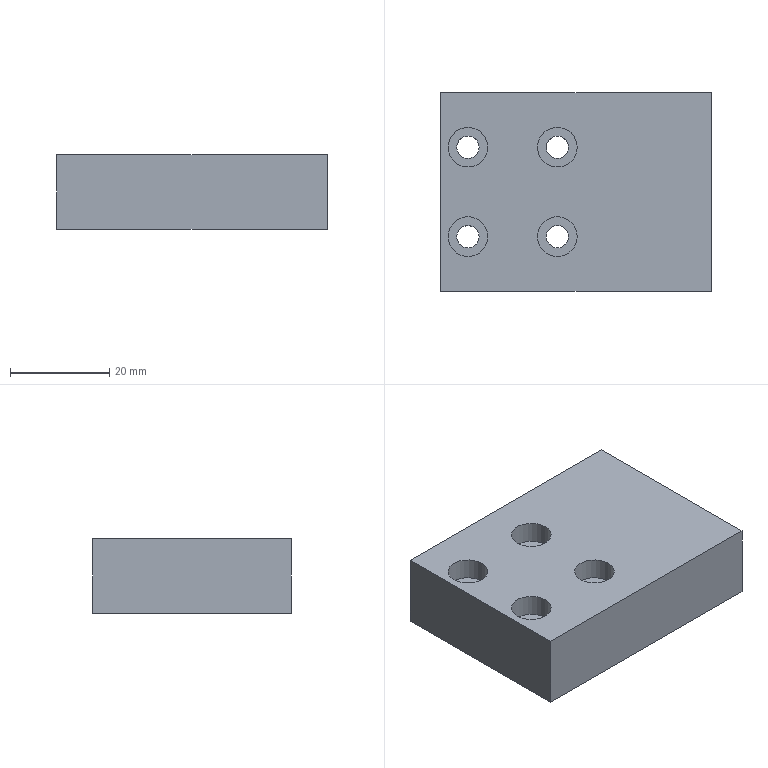Part | NX | features BREP 1 | 1 solid | 28 faces | box 54.5 x 40 x 15 mm | volume 29612 mm3 | cylinder 13 | plane 12 | cone 3 | commonest cylinder face diameters 4.5 x4 6 x4 8 x4 6.8 x1
STEP:
#1=CARTESIAN_POINT('',(-1.5,-9.,3.1));
#2=VERTEX_POINT('',#1);
#3=CARTESIAN_POINT('',(-3.75,-9.,3.1));
#4=DIRECTION('',(0.,0.,1.));
#5=DIRECTION('',(1.,0.,0.));
#6=AXIS2_PLACEMENT_3D('',#3,#4,#5);
#7=CIRCLE('',#6,2.25);
#8=EDGE_CURVE('',#2,#2,#7,.T.);
#9=ORIENTED_EDGE('',*,*,#8,.T.);
#10=EDGE_LOOP('',(#9));
#11=FACE_BOUND('',#10,.T.);
#12=CARTESIAN_POINT('',(-6.,-9.,-4.5));
#13=VERTEX_POINT('',#12);
#14=CARTESIAN_POINT('',(-3.75,-9.,-4.5));
#15=DIRECTION('',(0.,0.,1.));
#16=DIRECTION('',(-1.,0.,0.));
#17=AXIS2_PLACEMENT_3D('',#14,#15,#16);
#18=CIRCLE('',#17,2.25);
#19=EDGE_CURVE('',#13,#13,#18,.T.);
#20=ORIENTED_EDGE('',*,*,#19,.F.);
#21=EDGE_LOOP('',(#20));
#22=FACE_BOUND('',#21,.T.);
#23=CARTESIAN_POINT('',(-3.75,-9.,7.5));
#24=DIRECTION('',(0.,0.,1.));
#25=DIRECTION('',(-1.,0.,0.));
#26=AXIS2_PLACEMENT_3D('',#23,#24,#25);
#27=CYLINDRICAL_SURFACE('',#26,2.25);
#28=ADVANCED_FACE('',(#11,#22),#27,.F.);
#29=CARTESIAN_POINT('',(-19.5,9.,3.1));
#30=VERTEX_POINT('',#29);
#31=CARTESIAN_POINT('',(-21.75,9.,3.1));
#32=DIRECTION('',(0.,0.,1.));
#33=DIRECTION('',(1.,0.,0.));
#34=AXIS2_PLACEMENT_3D('',#31,#32,#33);
#35=CIRCLE('',#34,2.25);
#36=EDGE_CURVE('',#30,#30,#35,.T.);
#37=ORIENTED_EDGE('',*,*,#36,.T.);
#38=EDGE_LOOP('',(#37));
#39=FACE_BOUND('',#38,.T.);
#40=CARTESIAN_POINT('',(-24.,9.,-4.5));
#41=VERTEX_POINT('',#40);
#42=CARTESIAN_POINT('',(-21.75,9.,-4.5));
#43=DIRECTION('',(0.,0.,1.));
#44=DIRECTION('',(-1.,0.,0.));
#45=AXIS2_PLACEMENT_3D('',#42,#43,#44);
#46=CIRCLE('',#45,2.25);
#47=EDGE_CURVE('',#41,#41,#46,.T.);
#48=ORIENTED_EDGE('',*,*,#47,.F.);
#49=EDGE_LOOP('',(#48));
#50=FACE_BOUND('',#49,.T.);
#51=CARTESIAN_POINT('',(-21.75,9.,7.5));
#52=DIRECTION('',(0.,0.,1.));
#53=DIRECTION('',(-1.,0.,0.));
#54=AXIS2_PLACEMENT_3D('',#51,#52,#53);
#55=CYLINDRICAL_SURFACE('',#54,2.25);
#56=ADVANCED_FACE('',(#39,#50),#55,.F.);
#57=CARTESIAN_POINT('',(27.25,0.,-3.4));
#58=VERTEX_POINT('',#57);
#59=CARTESIAN_POINT('',(27.25,0.,0.));
#60=DIRECTION('',(1.,0.,0.));
#61=DIRECTION('',(0.,0.,-1.));
#62=AXIS2_PLACEMENT_3D('',#59,#60,#61);
#63=CIRCLE('',#62,3.4);
#64=EDGE_CURVE('',#58,#58,#63,.T.);
#65=ORIENTED_EDGE('',*,*,#64,.F.);
#66=EDGE_LOOP('',(#65));
#67=FACE_BOUND('',#66,.T.);
#68=CARTESIAN_POINT('',(27.25,15.,-3.));
#69=VERTEX_POINT('',#68);
#70=CARTESIAN_POINT('',(27.25,15.,0.));
#71=DIRECTION('',(1.,0.,0.));
#72=DIRECTION('',(0.,0.,-1.));
#73=AXIS2_PLACEMENT_3D('',#70,#71,#72);
#74=CIRCLE('',#73,3.);
#75=EDGE_CURVE('',#69,#69,#74,.T.);
#76=ORIENTED_EDGE('',*,*,#75,.F.);
#77=EDGE_LOOP('',(#76));
#78=FACE_BOUND('',#77,.T.);
#79=CARTESIAN_POINT('',(27.25,-15.,-3.));
#80=VERTEX_POINT('',#79);
#81=CARTESIAN_POINT('',(27.25,-15.,0.));
#82=DIRECTION('',(1.,0.,0.));
#83=DIRECTION('',(0.,0.,-1.));
#84=AXIS2_PLACEMENT_3D('',#81,#82,#83);
#85=CIRCLE('',#84,3.);
#86=EDGE_CURVE('',#80,#80,#85,.T.);
#87=ORIENTED_EDGE('',*,*,#86,.F.);
#88=EDGE_LOOP('',(#87));
#89=FACE_BOUND('',#88,.T.);
#90=CARTESIAN_POINT('',(27.25,-20.,-7.5));
#91=VERTEX_POINT('',#90);
#92=CARTESIAN_POINT('',(27.25,20.,-7.5));
#93=VERTEX_POINT('',#92);
#94=CARTESIAN_POINT('',(27.25,-20.,-7.5));
#95=DIRECTION('',(0.,1.,0.));
#96=VECTOR('',#95,1000.);
#97=LINE('',#94,#96);
#98=EDGE_CURVE('',#91,#93,#97,.T.);
#99=ORIENTED_EDGE('',*,*,#98,.T.);
#100=CARTESIAN_POINT('',(27.25,20.,7.5));
#101=VERTEX_POINT('',#100);
#102=CARTESIAN_POINT('',(27.25,20.,7.5));
#103=DIRECTION('',(0.,0.,-1.));
#104=VECTOR('',#103,1000.);
#105=LINE('',#102,#104);
#106=EDGE_CURVE('',#101,#93,#105,.T.);
#107=ORIENTED_EDGE('',*,*,#106,.F.);
#108=CARTESIAN_POINT('',(27.25,-20.,7.5));
#109=VERTEX_POINT('',#108);
#110=CARTESIAN_POINT('',(27.25,-20.,7.5));
#111=DIRECTION('',(0.,1.,0.));
#112=VECTOR('',#111,1000.);
#113=LINE('',#110,#112);
#114=EDGE_CURVE('',#109,#101,#113,.T.);
#115=ORIENTED_EDGE('',*,*,#114,.F.);
#116=CARTESIAN_POINT('',(27.25,-20.,7.5));
#117=DIRECTION('',(0.,0.,-1.));
#118=VECTOR('',#117,1000.);
#119=LINE('',#116,#118);
#120=EDGE_CURVE('',#109,#91,#119,.T.);
#121=ORIENTED_EDGE('',*,*,#120,.T.);
#122=EDGE_LOOP('',(#99,#107,#115,#121));
#123=FACE_BOUND('',#122,.T.);
#124=CARTESIAN_POINT('',(27.25,-20.,7.5));
#125=DIRECTION('',(-1.,0.,0.));
#126=DIRECTION('',(0.,0.,-1.));
#127=AXIS2_PLACEMENT_3D('',#124,#125,#126);
#128=PLANE('',#127);
#129=ADVANCED_FACE('',(#67,#78,#89,#123),#128,.F.);
#130=CARTESIAN_POINT('',(-27.25,20.,-7.5));
#131=VERTEX_POINT('',#130);
#132=CARTESIAN_POINT('',(-27.25,20.,-7.5));
#133=DIRECTION('',(-1.,0.,0.));
#134=VECTOR('',#133,1000.);
#135=LINE('',#132,#134);
#136=EDGE_CURVE('',#93,#131,#135,.T.);
#137=ORIENTED_EDGE('',*,*,#136,.T.);
#138=CARTESIAN_POINT('',(-27.25,20.,7.5));
#139=VERTEX_POINT('',#138);
#140=CARTESIAN_POINT('',(-27.25,20.,7.5));
#141=DIRECTION('',(0.,0.,-1.));
#142=VECTOR('',#141,1000.);
#143=LINE('',#140,#142);
#144=EDGE_CURVE('',#139,#131,#143,.T.);
#145=ORIENTED_EDGE('',*,*,#144,.F.);
#146=CARTESIAN_POINT('',(-27.25,20.,7.5));
#147=DIRECTION('',(-1.,0.,0.));
#148=VECTOR('',#147,1000.);
#149=LINE('',#146,#148);
#150=EDGE_CURVE('',#101,#139,#149,.T.);
#151=ORIENTED_EDGE('',*,*,#150,.F.);
#152=ORIENTED_EDGE('',*,*,#106,.T.);
#153=EDGE_LOOP('',(#137,#145,#151,#152));
#154=FACE_BOUND('',#153,.T.);
#155=CARTESIAN_POINT('',(-27.25,20.,7.5));
#156=DIRECTION('',(0.,-1.,0.));
#157=DIRECTION('',(0.,0.,1.));
#158=AXIS2_PLACEMENT_3D('',#155,#156,#157);
#159=PLANE('',#158);
#160=ADVANCED_FACE('',(#154),#159,.F.);
#161=CARTESIAN_POINT('',(-27.25,-20.,-7.5));
#162=VERTEX_POINT('',#161);
#163=CARTESIAN_POINT('',(-27.25,-20.,-7.5));
#164=DIRECTION('',(0.,-1.,0.));
#165=VECTOR('',#164,1000.);
#166=LINE('',#163,#165);
#167=EDGE_CURVE('',#131,#162,#166,.T.);
#168=ORIENTED_EDGE('',*,*,#167,.T.);
#169=CARTESIAN_POINT('',(-27.25,-20.,7.5));
#170=VERTEX_POINT('',#169);
#171=CARTESIAN_POINT('',(-27.25,-20.,7.5));
#172=DIRECTION('',(0.,0.,-1.));
#173=VECTOR('',#172,1000.);
#174=LINE('',#171,#173);
#175=EDGE_CURVE('',#170,#162,#174,.T.);
#176=ORIENTED_EDGE('',*,*,#175,.F.);
#177=CARTESIAN_POINT('',(-27.25,-20.,7.5));
#178=DIRECTION('',(0.,-1.,0.));
#179=VECTOR('',#178,1000.);
#180=LINE('',#177,#179);
#181=EDGE_CURVE('',#139,#170,#180,.T.);
#182=ORIENTED_EDGE('',*,*,#181,.F.);
#183=ORIENTED_EDGE('',*,*,#144,.T.);
#184=EDGE_LOOP('',(#168,#176,#182,#183));
#185=FACE_BOUND('',#184,.T.);
#186=CARTESIAN_POINT('',(-27.25,-20.,7.5));
#187=DIRECTION('',(1.,0.,0.));
#188=DIRECTION('',(0.,0.,1.));
#189=AXIS2_PLACEMENT_3D('',#186,#187,#188);
#190=PLANE('',#189);
#191=ADVANCED_FACE('',(#185),#190,.F.);
#192=CARTESIAN_POINT('',(-27.25,-20.,-7.5));
#193=DIRECTION('',(1.,0.,0.));
#194=VECTOR('',#193,1000.);
#195=LINE('',#192,#194);
#196=EDGE_CURVE('',#162,#91,#195,.T.);
#197=ORIENTED_EDGE('',*,*,#196,.T.);
#198=ORIENTED_EDGE('',*,*,#120,.F.);
#199=CARTESIAN_POINT('',(-27.25,-20.,7.5));
#200=DIRECTION('',(1.,0.,0.));
#201=VECTOR('',#200,1000.);
#202=LINE('',#199,#201);
#203=EDGE_CURVE('',#170,#109,#202,.T.);
#204=ORIENTED_EDGE('',*,*,#203,.F.);
#205=ORIENTED_EDGE('',*,*,#175,.T.);
#206=EDGE_LOOP('',(#197,#198,#204,#205));
#207=FACE_BOUND('',#206,.T.);
#208=CARTESIAN_POINT('',(-27.25,-20.,7.5));
#209=DIRECTION('',(0.,1.,0.));
#210=DIRECTION('',(0.,0.,-1.));
#211=AXIS2_PLACEMENT_3D('',#208,#209,#210);
#212=PLANE('',#211);
#213=ADVANCED_FACE('',(#207),#212,.F.);
#214=CARTESIAN_POINT('',(-17.75,9.,7.5));
#215=VERTEX_POINT('',#214);
#216=CARTESIAN_POINT('',(-21.75,9.,7.5));
#217=DIRECTION('',(0.,0.,1.));
#218=DIRECTION('',(1.,0.,0.));
#219=AXIS2_PLACEMENT_3D('',#216,#217,#218);
#220=CIRCLE('',#219,4.);
#221=EDGE_CURVE('',#215,#215,#220,.T.);
#222=ORIENTED_EDGE('',*,*,#221,.F.);
#223=EDGE_LOOP('',(#222));
#224=FACE_BOUND('',#223,.T.);
#225=CARTESIAN_POINT('',(0.25,-9.,7.5));
#226=VERTEX_POINT('',#225);
#227=CARTESIAN_POINT('',(-3.75,-9.,7.5));
#228=DIRECTION('',(0.,0.,1.));
#229=DIRECTION('',(1.,0.,0.));
#230=AXIS2_PLACEMENT_3D('',#227,#228,#229);
#231=CIRCLE('',#230,4.);
#232=EDGE_CURVE('',#226,#226,#231,.T.);
#233=ORIENTED_EDGE('',*,*,#232,.F.);
#234=EDGE_LOOP('',(#233));
#235=FACE_BOUND('',#234,.T.);
#236=CARTESIAN_POINT('',(-17.75,-9.,7.5));
#237=VERTEX_POINT('',#236);
#238=CARTESIAN_POINT('',(-21.75,-9.,7.5));
#239=DIRECTION('',(0.,0.,1.));
#240=DIRECTION('',(1.,0.,0.));
#241=AXIS2_PLACEMENT_3D('',#238,#239,#240);
#242=CIRCLE('',#241,4.);
#243=EDGE_CURVE('',#237,#237,#242,.T.);
#244=ORIENTED_EDGE('',*,*,#243,.F.);
#245=EDGE_LOOP('',(#244));
#246=FACE_BOUND('',#245,.T.);
#247=CARTESIAN_POINT('',(0.25,9.,7.5));
#248=VERTEX_POINT('',#247);
#249=CARTESIAN_POINT('',(-3.75,9.,7.5));
#250=DIRECTION('',(0.,0.,1.));
#251=DIRECTION('',(1.,0.,0.));
#252=AXIS2_PLACEMENT_3D('',#249,#250,#251);
#253=CIRCLE('',#252,4.);
#254=EDGE_CURVE('',#248,#248,#253,.T.);
#255=ORIENTED_EDGE('',*,*,#254,.F.);
#256=EDGE_LOOP('',(#255));
#257=FACE_BOUND('',#256,.T.);
#258=ORIENTED_EDGE('',*,*,#114,.T.);
#259=ORIENTED_EDGE('',*,*,#150,.T.);
#260=ORIENTED_EDGE('',*,*,#181,.T.);
#261=ORIENTED_EDGE('',*,*,#203,.T.);
#262=EDGE_LOOP('',(#258,#259,#260,#261));
#263=FACE_BOUND('',#262,.T.);
#264=CARTESIAN_POINT('',(0.,0.,7.5));
#265=DIRECTION('',(0.,0.,-1.));
#266=DIRECTION('',(1.,0.,0.));
#267=AXIS2_PLACEMENT_3D('',#264,#265,#266);
#268=PLANE('',#267);
#269=ADVANCED_FACE('',(#224,#235,#246,#257,#263),#268,.F.);
#270=CARTESIAN_POINT('',(-24.75,9.,-7.5));
#271=VERTEX_POINT('',#270);
#272=CARTESIAN_POINT('',(-21.75,9.,-7.5));
#273=DIRECTION('',(0.,0.,-1.));
#274=DIRECTION('',(-1.,0.,0.));
#275=AXIS2_PLACEMENT_3D('',#272,#273,#274);
#276=CIRCLE('',#275,3.);
#277=EDGE_CURVE('',#271,#271,#276,.T.);
#278=ORIENTED_EDGE('',*,*,#277,.F.);
#279=EDGE_LOOP('',(#278));
#280=FACE_BOUND('',#279,.T.);
#281=CARTESIAN_POINT('',(-6.75,-9.,-7.5));
#282=VERTEX_POINT('',#281);
#283=CARTESIAN_POINT('',(-3.75,-9.,-7.5));
#284=DIRECTION('',(0.,0.,-1.));
#285=DIRECTION('',(-1.,0.,0.));
#286=AXIS2_PLACEMENT_3D('',#283,#284,#285);
#287=CIRCLE('',#286,3.);
#288=EDGE_CURVE('',#282,#282,#287,.T.);
#289=ORIENTED_EDGE('',*,*,#288,.F.);
#290=EDGE_LOOP('',(#289));
#291=FACE_BOUND('',#290,.T.);
#292=CARTESIAN_POINT('',(-19.5,-9.,-7.5));
#293=VERTEX_POINT('',#292);
#294=CARTESIAN_POINT('',(-21.75,-9.,-7.5));
#295=DIRECTION('',(0.,0.,1.));
#296=DIRECTION('',(1.,0.,0.));
#297=AXIS2_PLACEMENT_3D('',#294,#295,#296);
#298=CIRCLE('',#297,2.25);
#299=EDGE_CURVE('',#293,#293,#298,.T.);
#300=ORIENTED_EDGE('',*,*,#299,.T.);
#301=EDGE_LOOP('',(#300));
#302=FACE_BOUND('',#301,.T.);
#303=CARTESIAN_POINT('',(-1.5,9.,-7.5));
#304=VERTEX_POINT('',#303);
#305=CARTESIAN_POINT('',(-3.75,9.,-7.5));
#306=DIRECTION('',(0.,0.,1.));
#307=DIRECTION('',(1.,0.,0.));
#308=AXIS2_PLACEMENT_3D('',#305,#306,#307);
#309=CIRCLE('',#308,2.25);
#310=EDGE_CURVE('',#304,#304,#309,.T.);
#311=ORIENTED_EDGE('',*,*,#310,.T.);
#312=EDGE_LOOP('',(#311));
#313=FACE_BOUND('',#312,.T.);
#314=ORIENTED_EDGE('',*,*,#98,.F.);
#315=ORIENTED_EDGE('',*,*,#196,.F.);
#316=ORIENTED_EDGE('',*,*,#167,.F.);
#317=ORIENTED_EDGE('',*,*,#136,.F.);
#318=EDGE_LOOP('',(#314,#315,#316,#317));
#319=FACE_BOUND('',#318,.T.);
#320=CARTESIAN_POINT('',(0.,0.,-7.5));
#321=DIRECTION('',(0.,0.,-1.));
#322=DIRECTION('',(1.,0.,0.));
#323=AXIS2_PLACEMENT_3D('',#320,#321,#322);
#324=PLANE('',#323);
#325=ADVANCED_FACE('',(#280,#291,#302,#313,#319),#324,.T.);
#326=ORIENTED_EDGE('',*,*,#310,.F.);
#327=EDGE_LOOP('',(#326));
#328=FACE_BOUND('',#327,.T.);
#329=CARTESIAN_POINT('',(-1.5,9.,3.1));
#330=VERTEX_POINT('',#329);
#331=CARTESIAN_POINT('',(-3.75,9.,3.1));
#332=DIRECTION('',(0.,0.,1.));
#333=DIRECTION('',(1.,0.,0.));
#334=AXIS2_PLACEMENT_3D('',#331,#332,#333);
#335=CIRCLE('',#334,2.25);
#336=EDGE_CURVE('',#330,#330,#335,.T.);
#337=ORIENTED_EDGE('',*,*,#336,.T.);
#338=EDGE_LOOP('',(#337));
#339=FACE_BOUND('',#338,.T.);
#340=CARTESIAN_POINT('',(-3.75,9.,7.5));
#341=DIRECTION('',(0.,0.,1.));
#342=DIRECTION('',(-1.,0.,0.));
#343=AXIS2_PLACEMENT_3D('',#340,#341,#342);
#344=CYLINDRICAL_SURFACE('',#343,2.25);
#345=ADVANCED_FACE('',(#328,#339),#344,.F.);
#346=ORIENTED_EDGE('',*,*,#336,.F.);
#347=EDGE_LOOP('',(#346));
#348=FACE_BOUND('',#347,.T.);
#349=CARTESIAN_POINT('',(0.25,9.,3.1));
#350=VERTEX_POINT('',#349);
#351=CARTESIAN_POINT('',(-3.75,9.,3.1));
#352=DIRECTION('',(0.,0.,1.));
#353=DIRECTION('',(1.,0.,0.));
#354=AXIS2_PLACEMENT_3D('',#351,#352,#353);
#355=CIRCLE('',#354,4.);
#356=EDGE_CURVE('',#350,#350,#355,.T.);
#357=ORIENTED_EDGE('',*,*,#356,.T.);
#358=EDGE_LOOP('',(#357));
#359=FACE_BOUND('',#358,.T.);
#360=CARTESIAN_POINT('',(-1.5,9.,3.1));
#361=DIRECTION('',(0.,0.,-1.));
#362=DIRECTION('',(1.,0.,0.));
#363=AXIS2_PLACEMENT_3D('',#360,#361,#362);
#364=PLANE('',#363);
#365=ADVANCED_FACE('',(#348,#359),#364,.F.);
#366=ORIENTED_EDGE('',*,*,#356,.F.);
#367=EDGE_LOOP('',(#366));
#368=FACE_BOUND('',#367,.T.);
#369=ORIENTED_EDGE('',*,*,#254,.T.);
#370=EDGE_LOOP('',(#369));
#371=FACE_BOUND('',#370,.T.);
#372=CARTESIAN_POINT('',(-3.75,9.,7.5));
#373=DIRECTION('',(0.,0.,1.));
#374=DIRECTION('',(-1.,0.,0.));
#375=AXIS2_PLACEMENT_3D('',#372,#373,#374);
#376=CYLINDRICAL_SURFACE('',#375,4.);
#377=ADVANCED_FACE('',(#368,#371),#376,.F.);
#378=ORIENTED_EDGE('',*,*,#299,.F.);
#379=EDGE_LOOP('',(#378));
#380=FACE_BOUND('',#379,.T.);
#381=CARTESIAN_POINT('',(-19.5,-9.,3.1));
#382=VERTEX_POINT('',#381);
#383=CARTESIAN_POINT('',(-21.75,-9.,3.1));
#384=DIRECTION('',(0.,0.,1.));
#385=DIRECTION('',(1.,0.,0.));
#386=AXIS2_PLACEMENT_3D('',#383,#384,#385);
#387=CIRCLE('',#386,2.25);
#388=EDGE_CURVE('',#382,#382,#387,.T.);
#389=ORIENTED_EDGE('',*,*,#388,.T.);
#390=EDGE_LOOP('',(#389));
#391=FACE_BOUND('',#390,.T.);
#392=CARTESIAN_POINT('',(-21.75,-9.,7.5));
#393=DIRECTION('',(0.,0.,1.));
#394=DIRECTION('',(-1.,0.,0.));
#395=AXIS2_PLACEMENT_3D('',#392,#393,#394);
#396=CYLINDRICAL_SURFACE('',#395,2.25);
#397=ADVANCED_FACE('',(#380,#391),#396,.F.);
#398=ORIENTED_EDGE('',*,*,#388,.F.);
#399=EDGE_LOOP('',(#398));
#400=FACE_BOUND('',#399,.T.);
#401=CARTESIAN_POINT('',(-17.75,-9.,3.1));
#402=VERTEX_POINT('',#401);
#403=CARTESIAN_POINT('',(-21.75,-9.,3.1));
#404=DIRECTION('',(0.,0.,1.));
#405=DIRECTION('',(1.,0.,0.));
#406=AXIS2_PLACEMENT_3D('',#403,#404,#405);
#407=CIRCLE('',#406,4.);
#408=EDGE_CURVE('',#402,#402,#407,.T.);
#409=ORIENTED_EDGE('',*,*,#408,.T.);
#410=EDGE_LOOP('',(#409));
#411=FACE_BOUND('',#410,.T.);
#412=CARTESIAN_POINT('',(-19.5,-9.,3.1));
#413=DIRECTION('',(0.,0.,-1.));
#414=DIRECTION('',(1.,0.,0.));
#415=AXIS2_PLACEMENT_3D('',#412,#413,#414);
#416=PLANE('',#415);
#417=ADVANCED_FACE('',(#400,#411),#416,.F.);
#418=ORIENTED_EDGE('',*,*,#408,.F.);
#419=EDGE_LOOP('',(#418));
#420=FACE_BOUND('',#419,.T.);
#421=ORIENTED_EDGE('',*,*,#243,.T.);
#422=EDGE_LOOP('',(#421));
#423=FACE_BOUND('',#422,.T.);
#424=CARTESIAN_POINT('',(-21.75,-9.,7.5));
#425=DIRECTION('',(0.,0.,1.));
#426=DIRECTION('',(-1.,0.,0.));
#427=AXIS2_PLACEMENT_3D('',#424,#425,#426);
#428=CYLINDRICAL_SURFACE('',#427,4.);
#429=ADVANCED_FACE('',(#420,#423),#428,.F.);
#430=ORIENTED_EDGE('',*,*,#8,.F.);
#431=EDGE_LOOP('',(#430));
#432=FACE_BOUND('',#431,.T.);
#433=CARTESIAN_POINT('',(0.25,-9.,3.1));
#434=VERTEX_POINT('',#433);
#435=CARTESIAN_POINT('',(-3.75,-9.,3.1));
#436=DIRECTION('',(0.,0.,1.));
#437=DIRECTION('',(1.,0.,0.));
#438=AXIS2_PLACEMENT_3D('',#435,#436,#437);
#439=CIRCLE('',#438,4.);
#440=EDGE_CURVE('',#434,#434,#439,.T.);
#441=ORIENTED_EDGE('',*,*,#440,.T.);
#442=EDGE_LOOP('',(#441));
#443=FACE_BOUND('',#442,.T.);
#444=CARTESIAN_POINT('',(-1.5,-9.,3.1));
#445=DIRECTION('',(0.,0.,-1.));
#446=DIRECTION('',(1.,0.,0.));
#447=AXIS2_PLACEMENT_3D('',#444,#445,#446);
#448=PLANE('',#447);
#449=ADVANCED_FACE('',(#432,#443),#448,.F.);
#450=ORIENTED_EDGE('',*,*,#440,.F.);
#451=EDGE_LOOP('',(#450));
#452=FACE_BOUND('',#451,.T.);
#453=ORIENTED_EDGE('',*,*,#232,.T.);
#454=EDGE_LOOP('',(#453));
#455=FACE_BOUND('',#454,.T.);
#456=CARTESIAN_POINT('',(-3.75,-9.,7.5));
#457=DIRECTION('',(0.,0.,1.));
#458=DIRECTION('',(-1.,0.,0.));
#459=AXIS2_PLACEMENT_3D('',#456,#457,#458);
#460=CYLINDRICAL_SURFACE('',#459,4.);
#461=ADVANCED_FACE('',(#452,#455),#460,.F.);
#462=ORIENTED_EDGE('',*,*,#36,.F.);
#463=EDGE_LOOP('',(#462));
#464=FACE_BOUND('',#463,.T.);
#465=CARTESIAN_POINT('',(-17.75,9.,3.1));
#466=VERTEX_POINT('',#465);
#467=CARTESIAN_POINT('',(-21.75,9.,3.1));
#468=DIRECTION('',(0.,0.,1.));
#469=DIRECTION('',(1.,0.,0.));
#470=AXIS2_PLACEMENT_3D('',#467,#468,#469);
#471=CIRCLE('',#470,4.);
#472=EDGE_CURVE('',#466,#466,#471,.T.);
#473=ORIENTED_EDGE('',*,*,#472,.T.);
#474=EDGE_LOOP('',(#473));
#475=FACE_BOUND('',#474,.T.);
#476=CARTESIAN_POINT('',(-19.5,9.,3.1));
#477=DIRECTION('',(0.,0.,-1.));
#478=DIRECTION('',(1.,0.,0.));
#479=AXIS2_PLACEMENT_3D('',#476,#477,#478);
#480=PLANE('',#479);
#481=ADVANCED_FACE('',(#464,#475),#480,.F.);
#482=ORIENTED_EDGE('',*,*,#472,.F.);
#483=EDGE_LOOP('',(#482));
#484=FACE_BOUND('',#483,.T.);
#485=ORIENTED_EDGE('',*,*,#221,.T.);
#486=EDGE_LOOP('',(#485));
#487=FACE_BOUND('',#486,.T.);
#488=CARTESIAN_POINT('',(-21.75,9.,7.5));
#489=DIRECTION('',(0.,0.,1.));
#490=DIRECTION('',(-1.,0.,0.));
#491=AXIS2_PLACEMENT_3D('',#488,#489,#490);
#492=CYLINDRICAL_SURFACE('',#491,4.);
#493=ADVANCED_FACE('',(#484,#487),#492,.F.);
#494=CARTESIAN_POINT('',(13.447,-15.,0.));
#495=VERTEX_POINT('',#494);
#496=VERTEX_LOOP('',#495);
#497=FACE_BOUND('',#496,.T.);
#498=CARTESIAN_POINT('',(15.25,-15.,-3.));
#499=VERTEX_POINT('',#498);
#500=CARTESIAN_POINT('',(15.25,-15.,0.));
#501=DIRECTION('',(1.,0.,0.));
#502=DIRECTION('',(0.,0.,-1.));
#503=AXIS2_PLACEMENT_3D('',#500,#501,#502);
#504=CIRCLE('',#503,3.);
#505=EDGE_CURVE('',#499,#499,#504,.T.);
#506=ORIENTED_EDGE('',*,*,#505,.T.);
#507=EDGE_LOOP('',(#506));
#508=FACE_BOUND('',#507,.T.);
#509=CARTESIAN_POINT('',(15.25,-15.,0.));
#510=DIRECTION('',(1.,0.,0.));
#511=DIRECTION('',(0.,0.,1.));
#512=AXIS2_PLACEMENT_3D('',#509,#510,#511);
#513=CONICAL_SURFACE('',#512,3.,1.03);
#514=ADVANCED_FACE('',(#497,#508),#513,.F.);
#515=ORIENTED_EDGE('',*,*,#505,.F.);
#516=EDGE_LOOP('',(#515));
#517=FACE_BOUND('',#516,.T.);
#518=ORIENTED_EDGE('',*,*,#86,.T.);
#519=EDGE_LOOP('',(#518));
#520=FACE_BOUND('',#519,.T.);
#521=CARTESIAN_POINT('',(27.25,-15.,0.));
#522=DIRECTION('',(1.,0.,0.));
#523=DIRECTION('',(0.,0.,1.));
#524=AXIS2_PLACEMENT_3D('',#521,#522,#523);
#525=CYLINDRICAL_SURFACE('',#524,3.);
#526=ADVANCED_FACE('',(#517,#520),#525,.F.);
#527=CARTESIAN_POINT('',(13.447,15.,0.));
#528=VERTEX_POINT('',#527);
#529=VERTEX_LOOP('',#528);
#530=FACE_BOUND('',#529,.T.);
#531=CARTESIAN_POINT('',(15.25,15.,-3.));
#532=VERTEX_POINT('',#531);
#533=CARTESIAN_POINT('',(15.25,15.,0.));
#534=DIRECTION('',(1.,0.,0.));
#535=DIRECTION('',(0.,0.,-1.));
#536=AXIS2_PLACEMENT_3D('',#533,#534,#535);
#537=CIRCLE('',#536,3.);
#538=EDGE_CURVE('',#532,#532,#537,.T.);
#539=ORIENTED_EDGE('',*,*,#538,.T.);
#540=EDGE_LOOP('',(#539));
#541=FACE_BOUND('',#540,.T.);
#542=CARTESIAN_POINT('',(15.25,15.,0.));
#543=DIRECTION('',(1.,0.,0.));
#544=DIRECTION('',(0.,0.,1.));
#545=AXIS2_PLACEMENT_3D('',#542,#543,#544);
#546=CONICAL_SURFACE('',#545,3.,1.03);
#547=ADVANCED_FACE('',(#530,#541),#546,.F.);
#548=ORIENTED_EDGE('',*,*,#538,.F.);
#549=EDGE_LOOP('',(#548));
#550=FACE_BOUND('',#549,.T.);
#551=ORIENTED_EDGE('',*,*,#75,.T.);
#552=EDGE_LOOP('',(#551));
#553=FACE_BOUND('',#552,.T.);
#554=CARTESIAN_POINT('',(27.25,15.,0.));
#555=DIRECTION('',(1.,0.,0.));
#556=DIRECTION('',(0.,0.,1.));
#557=AXIS2_PLACEMENT_3D('',#554,#555,#556);
#558=CYLINDRICAL_SURFACE('',#557,3.);
#559=ADVANCED_FACE('',(#550,#553),#558,.F.);
#560=CARTESIAN_POINT('',(5.457,0.,0.));
#561=VERTEX_POINT('',#560);
#562=VERTEX_LOOP('',#561);
#563=FACE_BOUND('',#562,.T.);
#564=CARTESIAN_POINT('',(7.5,0.,-3.4));
#565=VERTEX_POINT('',#564);
#566=CARTESIAN_POINT('',(7.5,0.,0.));
#567=DIRECTION('',(1.,0.,0.));
#568=DIRECTION('',(0.,0.,-1.));
#569=AXIS2_PLACEMENT_3D('',#566,#567,#568);
#570=CIRCLE('',#569,3.4);
#571=EDGE_CURVE('',#565,#565,#570,.T.);
#572=ORIENTED_EDGE('',*,*,#571,.T.);
#573=EDGE_LOOP('',(#572));
#574=FACE_BOUND('',#573,.T.);
#575=CARTESIAN_POINT('',(7.5,0.,0.));
#576=DIRECTION('',(1.,0.,0.));
#577=DIRECTION('',(0.,0.,1.));
#578=AXIS2_PLACEMENT_3D('',#575,#576,#577);
#579=CONICAL_SURFACE('',#578,3.4,1.03);
#580=ADVANCED_FACE('',(#563,#574),#579,.F.);
#581=ORIENTED_EDGE('',*,*,#571,.F.);
#582=EDGE_LOOP('',(#581));
#583=FACE_BOUND('',#582,.T.);
#584=ORIENTED_EDGE('',*,*,#64,.T.);
#585=EDGE_LOOP('',(#584));
#586=FACE_BOUND('',#585,.T.);
#587=CARTESIAN_POINT('',(27.25,0.,0.));
#588=DIRECTION('',(1.,0.,0.));
#589=DIRECTION('',(0.,0.,1.));
#590=AXIS2_PLACEMENT_3D('',#587,#588,#589);
#591=CYLINDRICAL_SURFACE('',#590,3.4);
#592=ADVANCED_FACE('',(#583,#586),#591,.F.);
#593=CARTESIAN_POINT('',(-24.75,9.,-4.5));
#594=VERTEX_POINT('',#593);
#595=CARTESIAN_POINT('',(-21.75,9.,-4.5));
#596=DIRECTION('',(0.,0.,-1.));
#597=DIRECTION('',(-1.,0.,0.));
#598=AXIS2_PLACEMENT_3D('',#595,#596,#597);
#599=CIRCLE('',#598,3.);
#600=EDGE_CURVE('',#594,#594,#599,.T.);
#601=ORIENTED_EDGE('',*,*,#600,.T.);
#602=EDGE_LOOP('',(#601));
#603=FACE_BOUND('',#602,.T.);
#604=ORIENTED_EDGE('',*,*,#47,.T.);
#605=EDGE_LOOP('',(#604));
#606=FACE_BOUND('',#605,.T.);
#607=CARTESIAN_POINT('',(-21.75,9.,-4.5));
#608=DIRECTION('',(0.,0.,-1.));
#609=DIRECTION('',(1.,0.,0.));
#610=AXIS2_PLACEMENT_3D('',#607,#608,#609);
#611=PLANE('',#610);
#612=ADVANCED_FACE('',(#603,#606),#611,.T.);
#613=ORIENTED_EDGE('',*,*,#600,.F.);
#614=EDGE_LOOP('',(#613));
#615=FACE_BOUND('',#614,.T.);
#616=ORIENTED_EDGE('',*,*,#277,.T.);
#617=EDGE_LOOP('',(#616));
#618=FACE_BOUND('',#617,.T.);
#619=CARTESIAN_POINT('',(-21.75,9.,-4.5));
#620=DIRECTION('',(0.,0.,-1.));
#621=DIRECTION('',(1.,0.,0.));
#622=AXIS2_PLACEMENT_3D('',#619,#620,#621);
#623=CYLINDRICAL_SURFACE('',#622,3.);
#624=ADVANCED_FACE('',(#615,#618),#623,.F.);
#625=CARTESIAN_POINT('',(-6.75,-9.,-4.5));
#626=VERTEX_POINT('',#625);
#627=CARTESIAN_POINT('',(-3.75,-9.,-4.5));
#628=DIRECTION('',(0.,0.,-1.));
#629=DIRECTION('',(-1.,0.,0.));
#630=AXIS2_PLACEMENT_3D('',#627,#628,#629);
#631=CIRCLE('',#630,3.);
#632=EDGE_CURVE('',#626,#626,#631,.T.);
#633=ORIENTED_EDGE('',*,*,#632,.T.);
#634=EDGE_LOOP('',(#633));
#635=FACE_BOUND('',#634,.T.);
#636=ORIENTED_EDGE('',*,*,#19,.T.);
#637=EDGE_LOOP('',(#636));
#638=FACE_BOUND('',#637,.T.);
#639=CARTESIAN_POINT('',(-3.75,-9.,-4.5));
#640=DIRECTION('',(0.,0.,-1.));
#641=DIRECTION('',(1.,0.,0.));
#642=AXIS2_PLACEMENT_3D('',#639,#640,#641);
#643=PLANE('',#642);
#644=ADVANCED_FACE('',(#635,#638),#643,.T.);
#645=ORIENTED_EDGE('',*,*,#632,.F.);
#646=EDGE_LOOP('',(#645));
#647=FACE_BOUND('',#646,.T.);
#648=ORIENTED_EDGE('',*,*,#288,.T.);
#649=EDGE_LOOP('',(#648));
#650=FACE_BOUND('',#649,.T.);
#651=CARTESIAN_POINT('',(-3.75,-9.,-4.5));
#652=DIRECTION('',(0.,0.,-1.));
#653=DIRECTION('',(1.,0.,0.));
#654=AXIS2_PLACEMENT_3D('',#651,#652,#653);
#655=CYLINDRICAL_SURFACE('',#654,3.);
#656=ADVANCED_FACE('',(#647,#650),#655,.F.);
#657=CLOSED_SHELL('',(#28,#56,#129,#160,#191,#213,#269,#325,#345,#365,#377,#397,#417,#429,#449,#461,#481,#493,#514,#526,#547,#559,#580,#592,#612,#624,#644,#656));
#658=MANIFOLD_SOLID_BREP('',#657);
#659=(LENGTH_UNIT()NAMED_UNIT(*)SI_UNIT(.MILLI.,.METRE.));
#660=UNCERTAINTY_MEASURE_WITH_UNIT(LENGTH_MEASURE(0.00001),#659,'','');
#661=(NAMED_UNIT(*)PLANE_ANGLE_UNIT()SI_UNIT($,.RADIAN.));
#662=(NAMED_UNIT(*)SI_UNIT($,.STERADIAN.)SOLID_ANGLE_UNIT());
#663=(GEOMETRIC_REPRESENTATION_CONTEXT(3)GLOBAL_UNCERTAINTY_ASSIGNED_CONTEXT((#660))GLOBAL_UNIT_ASSIGNED_CONTEXT((#659,#661,#662))REPRESENTATION_CONTEXT('',''));
#664=ADVANCED_BREP_SHAPE_REPRESENTATION('',(#658),#663);